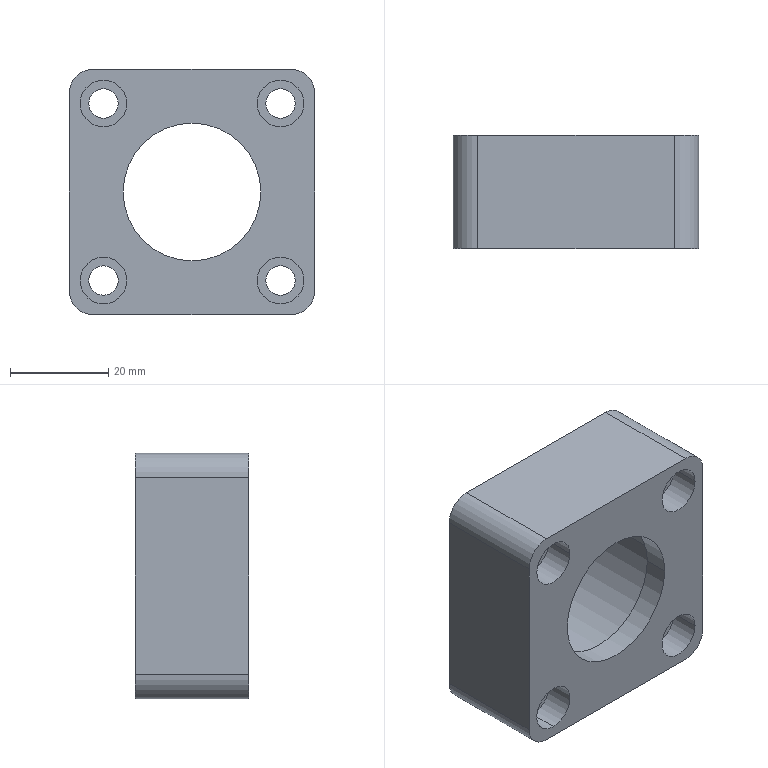Part | NX | features BREP 1 | 1 solid | 35 faces | box 50 x 23 x 50 mm | volume 32986 mm3 | cylinder 24 | plane 11 | commonest cylinder face diameters 6 x8 9.5 x8 10 x4 28 x2 35 x2
STEP:
#1=CARTESIAN_POINT('',(25.,0.,20.));
#2=VERTEX_POINT('',#1);
#3=CARTESIAN_POINT('',(25.,0.,-20.));
#4=VERTEX_POINT('',#3);
#5=CARTESIAN_POINT('',(25.,0.,20.));
#6=DIRECTION('',(0.,0.,-1.));
#7=VECTOR('',#6,1000.);
#8=LINE('',#5,#7);
#9=EDGE_CURVE('',#2,#4,#8,.T.);
#10=ORIENTED_EDGE('',*,*,#9,.F.);
#11=CARTESIAN_POINT('',(20.,0.,25.));
#12=VERTEX_POINT('',#11);
#13=CARTESIAN_POINT('',(20.,0.,20.));
#14=DIRECTION('',(0.,-1.,0.));
#15=DIRECTION('',(1.,0.,0.));
#16=AXIS2_PLACEMENT_3D('',#13,#14,#15);
#17=CIRCLE('',#16,5.);
#18=EDGE_CURVE('',#2,#12,#17,.T.);
#19=ORIENTED_EDGE('',*,*,#18,.T.);
#20=CARTESIAN_POINT('',(-20.,0.,25.));
#21=VERTEX_POINT('',#20);
#22=CARTESIAN_POINT('',(-20.,0.,25.));
#23=DIRECTION('',(1.,0.,0.));
#24=VECTOR('',#23,1000.);
#25=LINE('',#22,#24);
#26=EDGE_CURVE('',#21,#12,#25,.T.);
#27=ORIENTED_EDGE('',*,*,#26,.F.);
#28=CARTESIAN_POINT('',(-25.,0.,20.));
#29=VERTEX_POINT('',#28);
#30=CARTESIAN_POINT('',(-20.,0.,20.));
#31=DIRECTION('',(0.,-1.,0.));
#32=DIRECTION('',(0.,0.,1.));
#33=AXIS2_PLACEMENT_3D('',#30,#31,#32);
#34=CIRCLE('',#33,5.);
#35=EDGE_CURVE('',#21,#29,#34,.T.);
#36=ORIENTED_EDGE('',*,*,#35,.T.);
#37=CARTESIAN_POINT('',(-25.,0.,-20.));
#38=VERTEX_POINT('',#37);
#39=CARTESIAN_POINT('',(-25.,0.,-20.));
#40=DIRECTION('',(0.,0.,1.));
#41=VECTOR('',#40,1000.);
#42=LINE('',#39,#41);
#43=EDGE_CURVE('',#38,#29,#42,.T.);
#44=ORIENTED_EDGE('',*,*,#43,.F.);
#45=CARTESIAN_POINT('',(-20.,0.,-25.));
#46=VERTEX_POINT('',#45);
#47=CARTESIAN_POINT('',(-20.,0.,-20.));
#48=DIRECTION('',(0.,-1.,0.));
#49=DIRECTION('',(-1.,0.,0.));
#50=AXIS2_PLACEMENT_3D('',#47,#48,#49);
#51=CIRCLE('',#50,5.);
#52=EDGE_CURVE('',#38,#46,#51,.T.);
#53=ORIENTED_EDGE('',*,*,#52,.T.);
#54=CARTESIAN_POINT('',(20.,0.,-25.));
#55=VERTEX_POINT('',#54);
#56=CARTESIAN_POINT('',(20.,0.,-25.));
#57=DIRECTION('',(-1.,0.,0.));
#58=VECTOR('',#57,1000.);
#59=LINE('',#56,#58);
#60=EDGE_CURVE('',#55,#46,#59,.T.);
#61=ORIENTED_EDGE('',*,*,#60,.F.);
#62=CARTESIAN_POINT('',(20.,0.,-20.));
#63=DIRECTION('',(0.,-1.,0.));
#64=DIRECTION('',(0.,0.,-1.));
#65=AXIS2_PLACEMENT_3D('',#62,#63,#64);
#66=CIRCLE('',#65,5.);
#67=EDGE_CURVE('',#55,#4,#66,.T.);
#68=ORIENTED_EDGE('',*,*,#67,.T.);
#69=EDGE_LOOP('',(#10,#19,#27,#36,#44,#53,#61,#68));
#70=FACE_BOUND('',#69,.T.);
#71=CARTESIAN_POINT('',(22.75,0.,-18.));
#72=VERTEX_POINT('',#71);
#73=CARTESIAN_POINT('',(13.25,0.,-18.));
#74=VERTEX_POINT('',#73);
#75=CARTESIAN_POINT('',(18.,0.,-18.));
#76=DIRECTION('',(0.,-1.,0.));
#77=DIRECTION('',(1.,0.,0.));
#78=AXIS2_PLACEMENT_3D('',#75,#76,#77);
#79=CIRCLE('',#78,4.75);
#80=EDGE_CURVE('',#72,#74,#79,.T.);
#81=ORIENTED_EDGE('',*,*,#80,.F.);
#82=CARTESIAN_POINT('',(18.,0.,-18.));
#83=DIRECTION('',(0.,-1.,0.));
#84=DIRECTION('',(-1.,0.,0.));
#85=AXIS2_PLACEMENT_3D('',#82,#83,#84);
#86=CIRCLE('',#85,4.75);
#87=EDGE_CURVE('',#74,#72,#86,.T.);
#88=ORIENTED_EDGE('',*,*,#87,.F.);
#89=EDGE_LOOP('',(#81,#88));
#90=FACE_BOUND('',#89,.T.);
#91=CARTESIAN_POINT('',(-18.,0.,-22.75));
#92=VERTEX_POINT('',#91);
#93=CARTESIAN_POINT('',(-18.,0.,-13.25));
#94=VERTEX_POINT('',#93);
#95=CARTESIAN_POINT('',(-18.,0.,-18.));
#96=DIRECTION('',(0.,-1.,0.));
#97=DIRECTION('',(0.,0.,-1.));
#98=AXIS2_PLACEMENT_3D('',#95,#96,#97);
#99=CIRCLE('',#98,4.75);
#100=EDGE_CURVE('',#92,#94,#99,.T.);
#101=ORIENTED_EDGE('',*,*,#100,.F.);
#102=CARTESIAN_POINT('',(-18.,0.,-18.));
#103=DIRECTION('',(0.,-1.,0.));
#104=DIRECTION('',(0.,0.,1.));
#105=AXIS2_PLACEMENT_3D('',#102,#103,#104);
#106=CIRCLE('',#105,4.75);
#107=EDGE_CURVE('',#94,#92,#106,.T.);
#108=ORIENTED_EDGE('',*,*,#107,.F.);
#109=EDGE_LOOP('',(#101,#108));
#110=FACE_BOUND('',#109,.T.);
#111=CARTESIAN_POINT('',(-22.75,0.,18.));
#112=VERTEX_POINT('',#111);
#113=CARTESIAN_POINT('',(-13.25,0.,18.));
#114=VERTEX_POINT('',#113);
#115=CARTESIAN_POINT('',(-18.,0.,18.));
#116=DIRECTION('',(0.,-1.,0.));
#117=DIRECTION('',(-1.,0.,0.));
#118=AXIS2_PLACEMENT_3D('',#115,#116,#117);
#119=CIRCLE('',#118,4.75);
#120=EDGE_CURVE('',#112,#114,#119,.T.);
#121=ORIENTED_EDGE('',*,*,#120,.F.);
#122=CARTESIAN_POINT('',(-18.,0.,18.));
#123=DIRECTION('',(0.,-1.,0.));
#124=DIRECTION('',(1.,0.,0.));
#125=AXIS2_PLACEMENT_3D('',#122,#123,#124);
#126=CIRCLE('',#125,4.75);
#127=EDGE_CURVE('',#114,#112,#126,.T.);
#128=ORIENTED_EDGE('',*,*,#127,.F.);
#129=EDGE_LOOP('',(#121,#128));
#130=FACE_BOUND('',#129,.T.);
#131=CARTESIAN_POINT('',(13.25,0.,18.));
#132=VERTEX_POINT('',#131);
#133=CARTESIAN_POINT('',(22.75,0.,18.));
#134=VERTEX_POINT('',#133);
#135=CARTESIAN_POINT('',(18.,0.,18.));
#136=DIRECTION('',(0.,-1.,0.));
#137=DIRECTION('',(-1.,0.,0.));
#138=AXIS2_PLACEMENT_3D('',#135,#136,#137);
#139=CIRCLE('',#138,4.75);
#140=EDGE_CURVE('',#132,#134,#139,.T.);
#141=ORIENTED_EDGE('',*,*,#140,.F.);
#142=CARTESIAN_POINT('',(18.,0.,18.));
#143=DIRECTION('',(0.,-1.,0.));
#144=DIRECTION('',(1.,0.,0.));
#145=AXIS2_PLACEMENT_3D('',#142,#143,#144);
#146=CIRCLE('',#145,4.75);
#147=EDGE_CURVE('',#134,#132,#146,.T.);
#148=ORIENTED_EDGE('',*,*,#147,.F.);
#149=EDGE_LOOP('',(#141,#148));
#150=FACE_BOUND('',#149,.T.);
#151=CARTESIAN_POINT('',(-14.,0.,0.));
#152=VERTEX_POINT('',#151);
#153=CARTESIAN_POINT('',(14.,0.,0.));
#154=VERTEX_POINT('',#153);
#155=CARTESIAN_POINT('',(0.,0.,0.));
#156=DIRECTION('',(0.,1.,0.));
#157=DIRECTION('',(-1.,0.,0.));
#158=AXIS2_PLACEMENT_3D('',#155,#156,#157);
#159=CIRCLE('',#158,14.);
#160=EDGE_CURVE('',#152,#154,#159,.T.);
#161=ORIENTED_EDGE('',*,*,#160,.T.);
#162=CARTESIAN_POINT('',(0.,0.,0.));
#163=DIRECTION('',(0.,1.,0.));
#164=DIRECTION('',(1.,0.,0.));
#165=AXIS2_PLACEMENT_3D('',#162,#163,#164);
#166=CIRCLE('',#165,14.);
#167=EDGE_CURVE('',#154,#152,#166,.T.);
#168=ORIENTED_EDGE('',*,*,#167,.T.);
#169=EDGE_LOOP('',(#161,#168));
#170=FACE_BOUND('',#169,.T.);
#171=CARTESIAN_POINT('',(0.,0.,0.));
#172=DIRECTION('',(0.,1.,0.));
#173=DIRECTION('',(1.,0.,0.));
#174=AXIS2_PLACEMENT_3D('',#171,#172,#173);
#175=PLANE('',#174);
#176=ADVANCED_FACE('',(#70,#90,#110,#130,#150,#170),#175,.F.);
#177=CARTESIAN_POINT('',(-14.,5.,0.));
#178=VERTEX_POINT('',#177);
#179=CARTESIAN_POINT('',(-14.,5.,0.));
#180=DIRECTION('',(0.,-1.,0.));
#181=VECTOR('',#180,1000.);
#182=LINE('',#179,#181);
#183=EDGE_CURVE('',#178,#152,#182,.T.);
#184=ORIENTED_EDGE('',*,*,#183,.T.);
#185=ORIENTED_EDGE('',*,*,#167,.F.);
#186=CARTESIAN_POINT('',(14.,5.,0.));
#187=VERTEX_POINT('',#186);
#188=CARTESIAN_POINT('',(14.,5.,0.));
#189=DIRECTION('',(0.,-1.,0.));
#190=VECTOR('',#189,1000.);
#191=LINE('',#188,#190);
#192=EDGE_CURVE('',#187,#154,#191,.T.);
#193=ORIENTED_EDGE('',*,*,#192,.F.);
#194=CARTESIAN_POINT('',(0.,5.,0.));
#195=DIRECTION('',(0.,1.,0.));
#196=DIRECTION('',(1.,0.,0.));
#197=AXIS2_PLACEMENT_3D('',#194,#195,#196);
#198=CIRCLE('',#197,14.);
#199=EDGE_CURVE('',#187,#178,#198,.T.);
#200=ORIENTED_EDGE('',*,*,#199,.T.);
#201=EDGE_LOOP('',(#184,#185,#193,#200));
#202=FACE_BOUND('',#201,.T.);
#203=CARTESIAN_POINT('',(0.,23.,0.));
#204=DIRECTION('',(0.,1.,0.));
#205=DIRECTION('',(1.,0.,0.));
#206=AXIS2_PLACEMENT_3D('',#203,#204,#205);
#207=CYLINDRICAL_SURFACE('',#206,14.);
#208=ADVANCED_FACE('',(#202),#207,.F.);
#209=CARTESIAN_POINT('',(-17.5,5.,0.));
#210=VERTEX_POINT('',#209);
#211=CARTESIAN_POINT('',(17.5,5.,0.));
#212=VERTEX_POINT('',#211);
#213=CARTESIAN_POINT('',(0.,5.,0.));
#214=DIRECTION('',(0.,1.,0.));
#215=DIRECTION('',(-1.,0.,0.));
#216=AXIS2_PLACEMENT_3D('',#213,#214,#215);
#217=CIRCLE('',#216,17.5);
#218=EDGE_CURVE('',#210,#212,#217,.T.);
#219=ORIENTED_EDGE('',*,*,#218,.T.);
#220=CARTESIAN_POINT('',(0.,5.,0.));
#221=DIRECTION('',(0.,1.,0.));
#222=DIRECTION('',(1.,0.,0.));
#223=AXIS2_PLACEMENT_3D('',#220,#221,#222);
#224=CIRCLE('',#223,17.5);
#225=EDGE_CURVE('',#212,#210,#224,.T.);
#226=ORIENTED_EDGE('',*,*,#225,.T.);
#227=EDGE_LOOP('',(#219,#226));
#228=FACE_BOUND('',#227,.T.);
#229=CARTESIAN_POINT('',(0.,5.,0.));
#230=DIRECTION('',(0.,1.,0.));
#231=DIRECTION('',(-1.,0.,0.));
#232=AXIS2_PLACEMENT_3D('',#229,#230,#231);
#233=CIRCLE('',#232,14.);
#234=EDGE_CURVE('',#178,#187,#233,.T.);
#235=ORIENTED_EDGE('',*,*,#234,.F.);
#236=ORIENTED_EDGE('',*,*,#199,.F.);
#237=EDGE_LOOP('',(#235,#236));
#238=FACE_BOUND('',#237,.T.);
#239=CARTESIAN_POINT('',(0.,5.,0.));
#240=DIRECTION('',(0.,1.,0.));
#241=DIRECTION('',(1.,0.,0.));
#242=AXIS2_PLACEMENT_3D('',#239,#240,#241);
#243=PLANE('',#242);
#244=ADVANCED_FACE('',(#228,#238),#243,.T.);
#245=CARTESIAN_POINT('',(-17.5,23.,0.));
#246=VERTEX_POINT('',#245);
#247=CARTESIAN_POINT('',(-17.5,23.,0.));
#248=DIRECTION('',(0.,-1.,0.));
#249=VECTOR('',#248,1000.);
#250=LINE('',#247,#249);
#251=EDGE_CURVE('',#246,#210,#250,.T.);
#252=ORIENTED_EDGE('',*,*,#251,.T.);
#253=ORIENTED_EDGE('',*,*,#225,.F.);
#254=CARTESIAN_POINT('',(17.5,23.,0.));
#255=VERTEX_POINT('',#254);
#256=CARTESIAN_POINT('',(17.5,23.,0.));
#257=DIRECTION('',(0.,-1.,0.));
#258=VECTOR('',#257,1000.);
#259=LINE('',#256,#258);
#260=EDGE_CURVE('',#255,#212,#259,.T.);
#261=ORIENTED_EDGE('',*,*,#260,.F.);
#262=CARTESIAN_POINT('',(0.,23.,0.));
#263=DIRECTION('',(0.,1.,0.));
#264=DIRECTION('',(1.,0.,0.));
#265=AXIS2_PLACEMENT_3D('',#262,#263,#264);
#266=CIRCLE('',#265,17.5);
#267=EDGE_CURVE('',#255,#246,#266,.T.);
#268=ORIENTED_EDGE('',*,*,#267,.T.);
#269=EDGE_LOOP('',(#252,#253,#261,#268));
#270=FACE_BOUND('',#269,.T.);
#271=CARTESIAN_POINT('',(0.,23.,0.));
#272=DIRECTION('',(0.,1.,0.));
#273=DIRECTION('',(1.,0.,0.));
#274=AXIS2_PLACEMENT_3D('',#271,#272,#273);
#275=CYLINDRICAL_SURFACE('',#274,17.5);
#276=ADVANCED_FACE('',(#270),#275,.F.);
#277=CARTESIAN_POINT('',(20.,23.,-25.));
#278=VERTEX_POINT('',#277);
#279=CARTESIAN_POINT('',(-20.,23.,-25.));
#280=VERTEX_POINT('',#279);
#281=CARTESIAN_POINT('',(20.,23.,-25.));
#282=DIRECTION('',(-1.,0.,0.));
#283=VECTOR('',#282,1000.);
#284=LINE('',#281,#283);
#285=EDGE_CURVE('',#278,#280,#284,.T.);
#286=ORIENTED_EDGE('',*,*,#285,.T.);
#287=CARTESIAN_POINT('',(-25.,23.,-20.));
#288=VERTEX_POINT('',#287);
#289=CARTESIAN_POINT('',(-20.,23.,-20.));
#290=DIRECTION('',(0.,1.,0.));
#291=DIRECTION('',(0.,0.,-1.));
#292=AXIS2_PLACEMENT_3D('',#289,#290,#291);
#293=CIRCLE('',#292,5.);
#294=EDGE_CURVE('',#280,#288,#293,.T.);
#295=ORIENTED_EDGE('',*,*,#294,.T.);
#296=CARTESIAN_POINT('',(-25.,23.,20.));
#297=VERTEX_POINT('',#296);
#298=CARTESIAN_POINT('',(-25.,23.,-20.));
#299=DIRECTION('',(0.,0.,1.));
#300=VECTOR('',#299,1000.);
#301=LINE('',#298,#300);
#302=EDGE_CURVE('',#288,#297,#301,.T.);
#303=ORIENTED_EDGE('',*,*,#302,.T.);
#304=CARTESIAN_POINT('',(-20.,23.,25.));
#305=VERTEX_POINT('',#304);
#306=CARTESIAN_POINT('',(-20.,23.,20.));
#307=DIRECTION('',(0.,1.,0.));
#308=DIRECTION('',(-1.,0.,0.));
#309=AXIS2_PLACEMENT_3D('',#306,#307,#308);
#310=CIRCLE('',#309,5.);
#311=EDGE_CURVE('',#297,#305,#310,.T.);
#312=ORIENTED_EDGE('',*,*,#311,.T.);
#313=CARTESIAN_POINT('',(20.,23.,25.));
#314=VERTEX_POINT('',#313);
#315=CARTESIAN_POINT('',(-20.,23.,25.));
#316=DIRECTION('',(1.,0.,0.));
#317=VECTOR('',#316,1000.);
#318=LINE('',#315,#317);
#319=EDGE_CURVE('',#305,#314,#318,.T.);
#320=ORIENTED_EDGE('',*,*,#319,.T.);
#321=CARTESIAN_POINT('',(25.,23.,20.));
#322=VERTEX_POINT('',#321);
#323=CARTESIAN_POINT('',(20.,23.,20.));
#324=DIRECTION('',(0.,1.,0.));
#325=DIRECTION('',(0.,0.,1.));
#326=AXIS2_PLACEMENT_3D('',#323,#324,#325);
#327=CIRCLE('',#326,5.);
#328=EDGE_CURVE('',#314,#322,#327,.T.);
#329=ORIENTED_EDGE('',*,*,#328,.T.);
#330=CARTESIAN_POINT('',(25.,23.,-20.));
#331=VERTEX_POINT('',#330);
#332=CARTESIAN_POINT('',(25.,23.,20.));
#333=DIRECTION('',(0.,0.,-1.));
#334=VECTOR('',#333,1000.);
#335=LINE('',#332,#334);
#336=EDGE_CURVE('',#322,#331,#335,.T.);
#337=ORIENTED_EDGE('',*,*,#336,.T.);
#338=CARTESIAN_POINT('',(20.,23.,-20.));
#339=DIRECTION('',(0.,1.,0.));
#340=DIRECTION('',(1.,0.,0.));
#341=AXIS2_PLACEMENT_3D('',#338,#339,#340);
#342=CIRCLE('',#341,5.);
#343=EDGE_CURVE('',#331,#278,#342,.T.);
#344=ORIENTED_EDGE('',*,*,#343,.T.);
#345=EDGE_LOOP('',(#286,#295,#303,#312,#320,#329,#337,#344));
#346=FACE_BOUND('',#345,.T.);
#347=CARTESIAN_POINT('',(21.,23.,-18.));
#348=VERTEX_POINT('',#347);
#349=CARTESIAN_POINT('',(15.,23.,-18.));
#350=VERTEX_POINT('',#349);
#351=CARTESIAN_POINT('',(18.,23.,-18.));
#352=DIRECTION('',(0.,-1.,0.));
#353=DIRECTION('',(1.,0.,0.));
#354=AXIS2_PLACEMENT_3D('',#351,#352,#353);
#355=CIRCLE('',#354,3.);
#356=EDGE_CURVE('',#348,#350,#355,.T.);
#357=ORIENTED_EDGE('',*,*,#356,.T.);
#358=CARTESIAN_POINT('',(18.,23.,-18.));
#359=DIRECTION('',(0.,-1.,0.));
#360=DIRECTION('',(-1.,0.,0.));
#361=AXIS2_PLACEMENT_3D('',#358,#359,#360);
#362=CIRCLE('',#361,3.);
#363=EDGE_CURVE('',#350,#348,#362,.T.);
#364=ORIENTED_EDGE('',*,*,#363,.T.);
#365=EDGE_LOOP('',(#357,#364));
#366=FACE_BOUND('',#365,.T.);
#367=CARTESIAN_POINT('',(-18.,23.,-21.));
#368=VERTEX_POINT('',#367);
#369=CARTESIAN_POINT('',(-18.,23.,-15.));
#370=VERTEX_POINT('',#369);
#371=CARTESIAN_POINT('',(-18.,23.,-18.));
#372=DIRECTION('',(0.,-1.,0.));
#373=DIRECTION('',(0.,0.,-1.));
#374=AXIS2_PLACEMENT_3D('',#371,#372,#373);
#375=CIRCLE('',#374,3.);
#376=EDGE_CURVE('',#368,#370,#375,.T.);
#377=ORIENTED_EDGE('',*,*,#376,.T.);
#378=CARTESIAN_POINT('',(-18.,23.,-18.));
#379=DIRECTION('',(0.,-1.,0.));
#380=DIRECTION('',(0.,0.,1.));
#381=AXIS2_PLACEMENT_3D('',#378,#379,#380);
#382=CIRCLE('',#381,3.);
#383=EDGE_CURVE('',#370,#368,#382,.T.);
#384=ORIENTED_EDGE('',*,*,#383,.T.);
#385=EDGE_LOOP('',(#377,#384));
#386=FACE_BOUND('',#385,.T.);
#387=CARTESIAN_POINT('',(-21.,23.,18.));
#388=VERTEX_POINT('',#387);
#389=CARTESIAN_POINT('',(-15.,23.,18.));
#390=VERTEX_POINT('',#389);
#391=CARTESIAN_POINT('',(-18.,23.,18.));
#392=DIRECTION('',(0.,-1.,0.));
#393=DIRECTION('',(-1.,0.,0.));
#394=AXIS2_PLACEMENT_3D('',#391,#392,#393);
#395=CIRCLE('',#394,3.);
#396=EDGE_CURVE('',#388,#390,#395,.T.);
#397=ORIENTED_EDGE('',*,*,#396,.T.);
#398=CARTESIAN_POINT('',(-18.,23.,18.));
#399=DIRECTION('',(0.,-1.,0.));
#400=DIRECTION('',(1.,0.,0.));
#401=AXIS2_PLACEMENT_3D('',#398,#399,#400);
#402=CIRCLE('',#401,3.);
#403=EDGE_CURVE('',#390,#388,#402,.T.);
#404=ORIENTED_EDGE('',*,*,#403,.T.);
#405=EDGE_LOOP('',(#397,#404));
#406=FACE_BOUND('',#405,.T.);
#407=CARTESIAN_POINT('',(15.,23.,18.));
#408=VERTEX_POINT('',#407);
#409=CARTESIAN_POINT('',(21.,23.,18.));
#410=VERTEX_POINT('',#409);
#411=CARTESIAN_POINT('',(18.,23.,18.));
#412=DIRECTION('',(0.,-1.,0.));
#413=DIRECTION('',(-1.,0.,0.));
#414=AXIS2_PLACEMENT_3D('',#411,#412,#413);
#415=CIRCLE('',#414,3.);
#416=EDGE_CURVE('',#408,#410,#415,.T.);
#417=ORIENTED_EDGE('',*,*,#416,.T.);
#418=CARTESIAN_POINT('',(18.,23.,18.));
#419=DIRECTION('',(0.,-1.,0.));
#420=DIRECTION('',(1.,0.,0.));
#421=AXIS2_PLACEMENT_3D('',#418,#419,#420);
#422=CIRCLE('',#421,3.);
#423=EDGE_CURVE('',#410,#408,#422,.T.);
#424=ORIENTED_EDGE('',*,*,#423,.T.);
#425=EDGE_LOOP('',(#417,#424));
#426=FACE_BOUND('',#425,.T.);
#427=CARTESIAN_POINT('',(0.,23.,0.));
#428=DIRECTION('',(0.,1.,0.));
#429=DIRECTION('',(-1.,0.,0.));
#430=AXIS2_PLACEMENT_3D('',#427,#428,#429);
#431=CIRCLE('',#430,17.5);
#432=EDGE_CURVE('',#246,#255,#431,.T.);
#433=ORIENTED_EDGE('',*,*,#432,.F.);
#434=ORIENTED_EDGE('',*,*,#267,.F.);
#435=EDGE_LOOP('',(#433,#434));
#436=FACE_BOUND('',#435,.T.);
#437=CARTESIAN_POINT('',(0.,23.,0.));
#438=DIRECTION('',(0.,1.,0.));
#439=DIRECTION('',(1.,0.,0.));
#440=AXIS2_PLACEMENT_3D('',#437,#438,#439);
#441=PLANE('',#440);
#442=ADVANCED_FACE('',(#346,#366,#386,#406,#426,#436),#441,.T.);
#443=ORIENTED_EDGE('',*,*,#260,.T.);
#444=ORIENTED_EDGE('',*,*,#218,.F.);
#445=ORIENTED_EDGE('',*,*,#251,.F.);
#446=ORIENTED_EDGE('',*,*,#432,.T.);
#447=EDGE_LOOP('',(#443,#444,#445,#446));
#448=FACE_BOUND('',#447,.T.);
#449=CARTESIAN_POINT('',(0.,23.,0.));
#450=DIRECTION('',(0.,1.,0.));
#451=DIRECTION('',(1.,0.,0.));
#452=AXIS2_PLACEMENT_3D('',#449,#450,#451);
#453=CYLINDRICAL_SURFACE('',#452,17.5);
#454=ADVANCED_FACE('',(#448),#453,.F.);
#455=CARTESIAN_POINT('',(15.,6.,-18.));
#456=VERTEX_POINT('',#455);
#457=CARTESIAN_POINT('',(15.,23.,-18.));
#458=DIRECTION('',(0.,-1.,0.));
#459=VECTOR('',#458,1000.);
#460=LINE('',#457,#459);
#461=EDGE_CURVE('',#350,#456,#460,.T.);
#462=ORIENTED_EDGE('',*,*,#461,.T.);
#463=CARTESIAN_POINT('',(21.,6.,-18.));
#464=VERTEX_POINT('',#463);
#465=CARTESIAN_POINT('',(18.,6.,-18.));
#466=DIRECTION('',(0.,-1.,0.));
#467=DIRECTION('',(-1.,0.,0.));
#468=AXIS2_PLACEMENT_3D('',#465,#466,#467);
#469=CIRCLE('',#468,3.);
#470=EDGE_CURVE('',#456,#464,#469,.T.);
#471=ORIENTED_EDGE('',*,*,#470,.T.);
#472=CARTESIAN_POINT('',(21.,23.,-18.));
#473=DIRECTION('',(0.,-1.,0.));
#474=VECTOR('',#473,1000.);
#475=LINE('',#472,#474);
#476=EDGE_CURVE('',#348,#464,#475,.T.);
#477=ORIENTED_EDGE('',*,*,#476,.F.);
#478=ORIENTED_EDGE('',*,*,#363,.F.);
#479=EDGE_LOOP('',(#462,#471,#477,#478));
#480=FACE_BOUND('',#479,.T.);
#481=CARTESIAN_POINT('',(18.,33.393,-18.));
#482=DIRECTION('',(0.,-1.,0.));
#483=DIRECTION('',(-1.,0.,0.));
#484=AXIS2_PLACEMENT_3D('',#481,#482,#483);
#485=CYLINDRICAL_SURFACE('',#484,3.);
#486=ADVANCED_FACE('',(#480),#485,.F.);
#487=ORIENTED_EDGE('',*,*,#476,.T.);
#488=CARTESIAN_POINT('',(18.,6.,-18.));
#489=DIRECTION('',(0.,1.,0.));
#490=DIRECTION('',(-1.,0.,0.));
#491=AXIS2_PLACEMENT_3D('',#488,#489,#490);
#492=CIRCLE('',#491,3.);
#493=EDGE_CURVE('',#456,#464,#492,.T.);
#494=ORIENTED_EDGE('',*,*,#493,.F.);
#495=ORIENTED_EDGE('',*,*,#461,.F.);
#496=ORIENTED_EDGE('',*,*,#356,.F.);
#497=EDGE_LOOP('',(#487,#494,#495,#496));
#498=FACE_BOUND('',#497,.T.);
#499=CARTESIAN_POINT('',(18.,33.393,-18.));
#500=DIRECTION('',(0.,-1.,0.));
#501=DIRECTION('',(-1.,0.,0.));
#502=AXIS2_PLACEMENT_3D('',#499,#500,#501);
#503=CYLINDRICAL_SURFACE('',#502,3.);
#504=ADVANCED_FACE('',(#498),#503,.F.);
#505=CARTESIAN_POINT('',(13.25,6.,-18.));
#506=VERTEX_POINT('',#505);
#507=CARTESIAN_POINT('',(22.75,6.,-18.));
#508=VERTEX_POINT('',#507);
#509=CARTESIAN_POINT('',(18.,6.,-18.));
#510=DIRECTION('',(0.,1.,0.));
#511=DIRECTION('',(-1.,0.,0.));
#512=AXIS2_PLACEMENT_3D('',#509,#510,#511);
#513=CIRCLE('',#512,4.75);
#514=EDGE_CURVE('',#506,#508,#513,.T.);
#515=ORIENTED_EDGE('',*,*,#514,.F.);
#516=CARTESIAN_POINT('',(18.,6.,-18.));
#517=DIRECTION('',(0.,-1.,0.));
#518=DIRECTION('',(-1.,0.,0.));
#519=AXIS2_PLACEMENT_3D('',#516,#517,#518);
#520=CIRCLE('',#519,4.75);
#521=EDGE_CURVE('',#506,#508,#520,.T.);
#522=ORIENTED_EDGE('',*,*,#521,.T.);
#523=EDGE_LOOP('',(#515,#522));
#524=FACE_BOUND('',#523,.T.);
#525=ORIENTED_EDGE('',*,*,#470,.F.);
#526=ORIENTED_EDGE('',*,*,#493,.T.);
#527=EDGE_LOOP('',(#525,#526));
#528=FACE_BOUND('',#527,.T.);
#529=CARTESIAN_POINT('',(18.,6.,-18.));
#530=DIRECTION('',(0.,-1.,0.));
#531=DIRECTION('',(0.,0.,-1.));
#532=AXIS2_PLACEMENT_3D('',#529,#530,#531);
#533=PLANE('',#532);
#534=ADVANCED_FACE('',(#524,#528),#533,.T.);
#535=CARTESIAN_POINT('',(22.75,6.,-18.));
#536=DIRECTION('',(0.,-1.,0.));
#537=VECTOR('',#536,1000.);
#538=LINE('',#535,#537);
#539=EDGE_CURVE('',#72,#508,#538,.F.);
#540=ORIENTED_EDGE('',*,*,#539,.T.);
#541=ORIENTED_EDGE('',*,*,#521,.F.);
#542=CARTESIAN_POINT('',(13.25,6.,-18.));
#543=DIRECTION('',(0.,-1.,0.));
#544=VECTOR('',#543,1000.);
#545=LINE('',#542,#544);
#546=EDGE_CURVE('',#74,#506,#545,.F.);
#547=ORIENTED_EDGE('',*,*,#546,.F.);
#548=ORIENTED_EDGE('',*,*,#87,.T.);
#549=EDGE_LOOP('',(#540,#541,#547,#548));
#550=FACE_BOUND('',#549,.T.);
#551=CARTESIAN_POINT('',(18.,33.393,-18.));
#552=DIRECTION('',(0.,-1.,0.));
#553=DIRECTION('',(-1.,0.,0.));
#554=AXIS2_PLACEMENT_3D('',#551,#552,#553);
#555=CYLINDRICAL_SURFACE('',#554,4.75);
#556=ADVANCED_FACE('',(#550),#555,.F.);
#557=ORIENTED_EDGE('',*,*,#546,.T.);
#558=ORIENTED_EDGE('',*,*,#514,.T.);
#559=ORIENTED_EDGE('',*,*,#539,.F.);
#560=ORIENTED_EDGE('',*,*,#80,.T.);
#561=EDGE_LOOP('',(#557,#558,#559,#560));
#562=FACE_BOUND('',#561,.T.);
#563=CARTESIAN_POINT('',(18.,33.393,-18.));
#564=DIRECTION('',(0.,-1.,0.));
#565=DIRECTION('',(-1.,0.,0.));
#566=AXIS2_PLACEMENT_3D('',#563,#564,#565);
#567=CYLINDRICAL_SURFACE('',#566,4.75);
#568=ADVANCED_FACE('',(#562),#567,.F.);
#569=CARTESIAN_POINT('',(-18.,6.,-15.));
#570=VERTEX_POINT('',#569);
#571=CARTESIAN_POINT('',(-18.,23.,-15.));
#572=DIRECTION('',(0.,-1.,0.));
#573=VECTOR('',#572,1000.);
#574=LINE('',#571,#573);
#575=EDGE_CURVE('',#570,#370,#574,.F.);
#576=ORIENTED_EDGE('',*,*,#575,.F.);
#577=CARTESIAN_POINT('',(-18.,6.,-21.));
#578=VERTEX_POINT('',#577);
#579=CARTESIAN_POINT('',(-18.,6.,-18.));
#580=DIRECTION('',(0.,-1.,0.));
#581=DIRECTION('',(0.,0.,1.));
#582=AXIS2_PLACEMENT_3D('',#579,#580,#581);
#583=CIRCLE('',#582,3.);
#584=EDGE_CURVE('',#570,#578,#583,.T.);
#585=ORIENTED_EDGE('',*,*,#584,.T.);
#586=CARTESIAN_POINT('',(-18.,23.,-21.));
#587=DIRECTION('',(0.,-1.,0.));
#588=VECTOR('',#587,1000.);
#589=LINE('',#586,#588);
#590=EDGE_CURVE('',#578,#368,#589,.F.);
#591=ORIENTED_EDGE('',*,*,#590,.T.);
#592=ORIENTED_EDGE('',*,*,#383,.F.);
#593=EDGE_LOOP('',(#576,#585,#591,#592));
#594=FACE_BOUND('',#593,.T.);
#595=CARTESIAN_POINT('',(-18.,33.393,-18.));
#596=DIRECTION('',(0.,-1.,0.));
#597=DIRECTION('',(0.,0.,1.));
#598=AXIS2_PLACEMENT_3D('',#595,#596,#597);
#599=CYLINDRICAL_SURFACE('',#598,3.);
#600=ADVANCED_FACE('',(#594),#599,.F.);
#601=ORIENTED_EDGE('',*,*,#590,.F.);
#602=CARTESIAN_POINT('',(-18.,6.,-18.));
#603=DIRECTION('',(0.,1.,0.));
#604=DIRECTION('',(0.,0.,1.));
#605=AXIS2_PLACEMENT_3D('',#602,#603,#604);
#606=CIRCLE('',#605,3.);
#607=EDGE_CURVE('',#570,#578,#606,.T.);
#608=ORIENTED_EDGE('',*,*,#607,.F.);
#609=ORIENTED_EDGE('',*,*,#575,.T.);
#610=ORIENTED_EDGE('',*,*,#376,.F.);
#611=EDGE_LOOP('',(#601,#608,#609,#610));
#612=FACE_BOUND('',#611,.T.);
#613=CARTESIAN_POINT('',(-18.,33.393,-18.));
#614=DIRECTION('',(0.,-1.,0.));
#615=DIRECTION('',(0.,0.,1.));
#616=AXIS2_PLACEMENT_3D('',#613,#614,#615);
#617=CYLINDRICAL_SURFACE('',#616,3.);
#618=ADVANCED_FACE('',(#612),#617,.F.);
#619=CARTESIAN_POINT('',(-18.,6.,-13.25));
#620=VERTEX_POINT('',#619);
#621=CARTESIAN_POINT('',(-18.,6.,-22.75));
#622=VERTEX_POINT('',#621);
#623=CARTESIAN_POINT('',(-18.,6.,-18.));
#624=DIRECTION('',(0.,1.,0.));
#625=DIRECTION('',(0.,0.,1.));
#626=AXIS2_PLACEMENT_3D('',#623,#624,#625);
#627=CIRCLE('',#626,4.75);
#628=EDGE_CURVE('',#620,#622,#627,.T.);
#629=ORIENTED_EDGE('',*,*,#628,.F.);
#630=CARTESIAN_POINT('',(-18.,6.,-18.));
#631=DIRECTION('',(0.,-1.,0.));
#632=DIRECTION('',(0.,0.,1.));
#633=AXIS2_PLACEMENT_3D('',#630,#631,#632);
#634=CIRCLE('',#633,4.75);
#635=EDGE_CURVE('',#620,#622,#634,.T.);
#636=ORIENTED_EDGE('',*,*,#635,.T.);
#637=EDGE_LOOP('',(#629,#636));
#638=FACE_BOUND('',#637,.T.);
#639=ORIENTED_EDGE('',*,*,#584,.F.);
#640=ORIENTED_EDGE('',*,*,#607,.T.);
#641=EDGE_LOOP('',(#639,#640));
#642=FACE_BOUND('',#641,.T.);
#643=CARTESIAN_POINT('',(-18.,6.,-18.));
#644=DIRECTION('',(0.,-1.,0.));
#645=DIRECTION('',(0.,0.,-1.));
#646=AXIS2_PLACEMENT_3D('',#643,#644,#645);
#647=PLANE('',#646);
#648=ADVANCED_FACE('',(#638,#642),#647,.T.);
#649=CARTESIAN_POINT('',(-18.,6.,-22.75));
#650=DIRECTION('',(0.,-1.,0.));
#651=VECTOR('',#650,1000.);
#652=LINE('',#649,#651);
#653=EDGE_CURVE('',#622,#92,#652,.T.);
#654=ORIENTED_EDGE('',*,*,#653,.F.);
#655=ORIENTED_EDGE('',*,*,#635,.F.);
#656=CARTESIAN_POINT('',(-18.,6.,-13.25));
#657=DIRECTION('',(0.,-1.,0.));
#658=VECTOR('',#657,1000.);
#659=LINE('',#656,#658);
#660=EDGE_CURVE('',#620,#94,#659,.T.);
#661=ORIENTED_EDGE('',*,*,#660,.T.);
#662=ORIENTED_EDGE('',*,*,#107,.T.);
#663=EDGE_LOOP('',(#654,#655,#661,#662));
#664=FACE_BOUND('',#663,.T.);
#665=CARTESIAN_POINT('',(-18.,33.393,-18.));
#666=DIRECTION('',(0.,-1.,0.));
#667=DIRECTION('',(0.,0.,1.));
#668=AXIS2_PLACEMENT_3D('',#665,#666,#667);
#669=CYLINDRICAL_SURFACE('',#668,4.75);
#670=ADVANCED_FACE('',(#664),#669,.F.);
#671=ORIENTED_EDGE('',*,*,#660,.F.);
#672=ORIENTED_EDGE('',*,*,#628,.T.);
#673=ORIENTED_EDGE('',*,*,#653,.T.);
#674=ORIENTED_EDGE('',*,*,#100,.T.);
#675=EDGE_LOOP('',(#671,#672,#673,#674));
#676=FACE_BOUND('',#675,.T.);
#677=CARTESIAN_POINT('',(-18.,33.393,-18.));
#678=DIRECTION('',(0.,-1.,0.));
#679=DIRECTION('',(0.,0.,1.));
#680=AXIS2_PLACEMENT_3D('',#677,#678,#679);
#681=CYLINDRICAL_SURFACE('',#680,4.75);
#682=ADVANCED_FACE('',(#676),#681,.F.);
#683=CARTESIAN_POINT('',(-15.,6.,18.));
#684=VERTEX_POINT('',#683);
#685=CARTESIAN_POINT('',(-15.,23.,18.));
#686=DIRECTION('',(0.,-1.,0.));
#687=VECTOR('',#686,1000.);
#688=LINE('',#685,#687);
#689=EDGE_CURVE('',#684,#390,#688,.F.);
#690=ORIENTED_EDGE('',*,*,#689,.F.);
#691=CARTESIAN_POINT('',(-21.,6.,18.));
#692=VERTEX_POINT('',#691);
#693=CARTESIAN_POINT('',(-18.,6.,18.));
#694=DIRECTION('',(0.,-1.,0.));
#695=DIRECTION('',(1.,0.,0.));
#696=AXIS2_PLACEMENT_3D('',#693,#694,#695);
#697=CIRCLE('',#696,3.);
#698=EDGE_CURVE('',#684,#692,#697,.T.);
#699=ORIENTED_EDGE('',*,*,#698,.T.);
#700=CARTESIAN_POINT('',(-21.,23.,18.));
#701=DIRECTION('',(0.,-1.,0.));
#702=VECTOR('',#701,1000.);
#703=LINE('',#700,#702);
#704=EDGE_CURVE('',#692,#388,#703,.F.);
#705=ORIENTED_EDGE('',*,*,#704,.T.);
#706=ORIENTED_EDGE('',*,*,#403,.F.);
#707=EDGE_LOOP('',(#690,#699,#705,#706));
#708=FACE_BOUND('',#707,.T.);
#709=CARTESIAN_POINT('',(-18.,33.393,18.));
#710=DIRECTION('',(0.,-1.,0.));
#711=DIRECTION('',(1.,0.,0.));
#712=AXIS2_PLACEMENT_3D('',#709,#710,#711);
#713=CYLINDRICAL_SURFACE('',#712,3.);
#714=ADVANCED_FACE('',(#708),#713,.F.);
#715=ORIENTED_EDGE('',*,*,#704,.F.);
#716=CARTESIAN_POINT('',(-18.,6.,18.));
#717=DIRECTION('',(0.,1.,0.));
#718=DIRECTION('',(1.,0.,0.));
#719=AXIS2_PLACEMENT_3D('',#716,#717,#718);
#720=CIRCLE('',#719,3.);
#721=EDGE_CURVE('',#684,#692,#720,.T.);
#722=ORIENTED_EDGE('',*,*,#721,.F.);
#723=ORIENTED_EDGE('',*,*,#689,.T.);
#724=ORIENTED_EDGE('',*,*,#396,.F.);
#725=EDGE_LOOP('',(#715,#722,#723,#724));
#726=FACE_BOUND('',#725,.T.);
#727=CARTESIAN_POINT('',(-18.,33.393,18.));
#728=DIRECTION('',(0.,-1.,0.));
#729=DIRECTION('',(1.,0.,0.));
#730=AXIS2_PLACEMENT_3D('',#727,#728,#729);
#731=CYLINDRICAL_SURFACE('',#730,3.);
#732=ADVANCED_FACE('',(#726),#731,.F.);
#733=CARTESIAN_POINT('',(-13.25,6.,18.));
#734=VERTEX_POINT('',#733);
#735=CARTESIAN_POINT('',(-22.75,6.,18.));
#736=VERTEX_POINT('',#735);
#737=CARTESIAN_POINT('',(-18.,6.,18.));
#738=DIRECTION('',(0.,1.,0.));
#739=DIRECTION('',(1.,0.,0.));
#740=AXIS2_PLACEMENT_3D('',#737,#738,#739);
#741=CIRCLE('',#740,4.75);
#742=EDGE_CURVE('',#734,#736,#741,.T.);
#743=ORIENTED_EDGE('',*,*,#742,.F.);
#744=CARTESIAN_POINT('',(-18.,6.,18.));
#745=DIRECTION('',(0.,-1.,0.));
#746=DIRECTION('',(1.,0.,0.));
#747=AXIS2_PLACEMENT_3D('',#744,#745,#746);
#748=CIRCLE('',#747,4.75);
#749=EDGE_CURVE('',#734,#736,#748,.T.);
#750=ORIENTED_EDGE('',*,*,#749,.T.);
#751=EDGE_LOOP('',(#743,#750));
#752=FACE_BOUND('',#751,.T.);
#753=ORIENTED_EDGE('',*,*,#698,.F.);
#754=ORIENTED_EDGE('',*,*,#721,.T.);
#755=EDGE_LOOP('',(#753,#754));
#756=FACE_BOUND('',#755,.T.);
#757=CARTESIAN_POINT('',(-18.,6.,18.));
#758=DIRECTION('',(0.,-1.,0.));
#759=DIRECTION('',(0.,0.,-1.));
#760=AXIS2_PLACEMENT_3D('',#757,#758,#759);
#761=PLANE('',#760);
#762=ADVANCED_FACE('',(#752,#756),#761,.T.);
#763=CARTESIAN_POINT('',(-22.75,6.,18.));
#764=DIRECTION('',(0.,-1.,0.));
#765=VECTOR('',#764,1000.);
#766=LINE('',#763,#765);
#767=EDGE_CURVE('',#736,#112,#766,.T.);
#768=ORIENTED_EDGE('',*,*,#767,.F.);
#769=ORIENTED_EDGE('',*,*,#749,.F.);
#770=CARTESIAN_POINT('',(-13.25,6.,18.));
#771=DIRECTION('',(0.,-1.,0.));
#772=VECTOR('',#771,1000.);
#773=LINE('',#770,#772);
#774=EDGE_CURVE('',#734,#114,#773,.T.);
#775=ORIENTED_EDGE('',*,*,#774,.T.);
#776=ORIENTED_EDGE('',*,*,#127,.T.);
#777=EDGE_LOOP('',(#768,#769,#775,#776));
#778=FACE_BOUND('',#777,.T.);
#779=CARTESIAN_POINT('',(-18.,33.393,18.));
#780=DIRECTION('',(0.,-1.,0.));
#781=DIRECTION('',(1.,0.,0.));
#782=AXIS2_PLACEMENT_3D('',#779,#780,#781);
#783=CYLINDRICAL_SURFACE('',#782,4.75);
#784=ADVANCED_FACE('',(#778),#783,.F.);
#785=ORIENTED_EDGE('',*,*,#774,.F.);
#786=ORIENTED_EDGE('',*,*,#742,.T.);
#787=ORIENTED_EDGE('',*,*,#767,.T.);
#788=ORIENTED_EDGE('',*,*,#120,.T.);
#789=EDGE_LOOP('',(#785,#786,#787,#788));
#790=FACE_BOUND('',#789,.T.);
#791=CARTESIAN_POINT('',(-18.,33.393,18.));
#792=DIRECTION('',(0.,-1.,0.));
#793=DIRECTION('',(1.,0.,0.));
#794=AXIS2_PLACEMENT_3D('',#791,#792,#793);
#795=CYLINDRICAL_SURFACE('',#794,4.75);
#796=ADVANCED_FACE('',(#790),#795,.F.);
#797=CARTESIAN_POINT('',(21.,6.,18.));
#798=VERTEX_POINT('',#797);
#799=CARTESIAN_POINT('',(21.,23.,18.));
#800=DIRECTION('',(0.,-1.,0.));
#801=VECTOR('',#800,1000.);
#802=LINE('',#799,#801);
#803=EDGE_CURVE('',#798,#410,#802,.F.);
#804=ORIENTED_EDGE('',*,*,#803,.F.);
#805=CARTESIAN_POINT('',(15.,6.,18.));
#806=VERTEX_POINT('',#805);
#807=CARTESIAN_POINT('',(18.,6.,18.));
#808=DIRECTION('',(0.,-1.,0.));
#809=DIRECTION('',(1.,0.,0.));
#810=AXIS2_PLACEMENT_3D('',#807,#808,#809);
#811=CIRCLE('',#810,3.);
#812=EDGE_CURVE('',#798,#806,#811,.T.);
#813=ORIENTED_EDGE('',*,*,#812,.T.);
#814=CARTESIAN_POINT('',(15.,23.,18.));
#815=DIRECTION('',(0.,-1.,0.));
#816=VECTOR('',#815,1000.);
#817=LINE('',#814,#816);
#818=EDGE_CURVE('',#806,#408,#817,.F.);
#819=ORIENTED_EDGE('',*,*,#818,.T.);
#820=ORIENTED_EDGE('',*,*,#423,.F.);
#821=EDGE_LOOP('',(#804,#813,#819,#820));
#822=FACE_BOUND('',#821,.T.);
#823=CARTESIAN_POINT('',(18.,33.393,18.));
#824=DIRECTION('',(0.,-1.,0.));
#825=DIRECTION('',(1.,0.,0.));
#826=AXIS2_PLACEMENT_3D('',#823,#824,#825);
#827=CYLINDRICAL_SURFACE('',#826,3.);
#828=ADVANCED_FACE('',(#822),#827,.F.);
#829=ORIENTED_EDGE('',*,*,#818,.F.);
#830=CARTESIAN_POINT('',(18.,6.,18.));
#831=DIRECTION('',(0.,1.,0.));
#832=DIRECTION('',(1.,0.,0.));
#833=AXIS2_PLACEMENT_3D('',#830,#831,#832);
#834=CIRCLE('',#833,3.);
#835=EDGE_CURVE('',#798,#806,#834,.T.);
#836=ORIENTED_EDGE('',*,*,#835,.F.);
#837=ORIENTED_EDGE('',*,*,#803,.T.);
#838=ORIENTED_EDGE('',*,*,#416,.F.);
#839=EDGE_LOOP('',(#829,#836,#837,#838));
#840=FACE_BOUND('',#839,.T.);
#841=CARTESIAN_POINT('',(18.,33.393,18.));
#842=DIRECTION('',(0.,-1.,0.));
#843=DIRECTION('',(1.,0.,0.));
#844=AXIS2_PLACEMENT_3D('',#841,#842,#843);
#845=CYLINDRICAL_SURFACE('',#844,3.);
#846=ADVANCED_FACE('',(#840),#845,.F.);
#847=CARTESIAN_POINT('',(22.75,6.,18.));
#848=VERTEX_POINT('',#847);
#849=CARTESIAN_POINT('',(13.25,6.,18.));
#850=VERTEX_POINT('',#849);
#851=CARTESIAN_POINT('',(18.,6.,18.));
#852=DIRECTION('',(0.,1.,0.));
#853=DIRECTION('',(1.,0.,0.));
#854=AXIS2_PLACEMENT_3D('',#851,#852,#853);
#855=CIRCLE('',#854,4.75);
#856=EDGE_CURVE('',#848,#850,#855,.T.);
#857=ORIENTED_EDGE('',*,*,#856,.F.);
#858=CARTESIAN_POINT('',(18.,6.,18.));
#859=DIRECTION('',(0.,-1.,0.));
#860=DIRECTION('',(1.,0.,0.));
#861=AXIS2_PLACEMENT_3D('',#858,#859,#860);
#862=CIRCLE('',#861,4.75);
#863=EDGE_CURVE('',#848,#850,#862,.T.);
#864=ORIENTED_EDGE('',*,*,#863,.T.);
#865=EDGE_LOOP('',(#857,#864));
#866=FACE_BOUND('',#865,.T.);
#867=ORIENTED_EDGE('',*,*,#812,.F.);
#868=ORIENTED_EDGE('',*,*,#835,.T.);
#869=EDGE_LOOP('',(#867,#868));
#870=FACE_BOUND('',#869,.T.);
#871=CARTESIAN_POINT('',(18.,6.,18.));
#872=DIRECTION('',(0.,-1.,0.));
#873=DIRECTION('',(0.,0.,-1.));
#874=AXIS2_PLACEMENT_3D('',#871,#872,#873);
#875=PLANE('',#874);
#876=ADVANCED_FACE('',(#866,#870),#875,.T.);
#877=CARTESIAN_POINT('',(13.25,6.,18.));
#878=DIRECTION('',(0.,-1.,0.));
#879=VECTOR('',#878,1000.);
#880=LINE('',#877,#879);
#881=EDGE_CURVE('',#850,#132,#880,.T.);
#882=ORIENTED_EDGE('',*,*,#881,.F.);
#883=ORIENTED_EDGE('',*,*,#863,.F.);
#884=CARTESIAN_POINT('',(22.75,6.,18.));
#885=DIRECTION('',(0.,-1.,0.));
#886=VECTOR('',#885,1000.);
#887=LINE('',#884,#886);
#888=EDGE_CURVE('',#848,#134,#887,.T.);
#889=ORIENTED_EDGE('',*,*,#888,.T.);
#890=ORIENTED_EDGE('',*,*,#147,.T.);
#891=EDGE_LOOP('',(#882,#883,#889,#890));
#892=FACE_BOUND('',#891,.T.);
#893=CARTESIAN_POINT('',(18.,33.393,18.));
#894=DIRECTION('',(0.,-1.,0.));
#895=DIRECTION('',(1.,0.,0.));
#896=AXIS2_PLACEMENT_3D('',#893,#894,#895);
#897=CYLINDRICAL_SURFACE('',#896,4.75);
#898=ADVANCED_FACE('',(#892),#897,.F.);
#899=ORIENTED_EDGE('',*,*,#888,.F.);
#900=ORIENTED_EDGE('',*,*,#856,.T.);
#901=ORIENTED_EDGE('',*,*,#881,.T.);
#902=ORIENTED_EDGE('',*,*,#140,.T.);
#903=EDGE_LOOP('',(#899,#900,#901,#902));
#904=FACE_BOUND('',#903,.T.);
#905=CARTESIAN_POINT('',(18.,33.393,18.));
#906=DIRECTION('',(0.,-1.,0.));
#907=DIRECTION('',(1.,0.,0.));
#908=AXIS2_PLACEMENT_3D('',#905,#906,#907);
#909=CYLINDRICAL_SURFACE('',#908,4.75);
#910=ADVANCED_FACE('',(#904),#909,.F.);
#911=CARTESIAN_POINT('',(20.,23.,-25.));
#912=DIRECTION('',(0.,-1.,0.));
#913=VECTOR('',#912,1000.);
#914=LINE('',#911,#913);
#915=EDGE_CURVE('',#278,#55,#914,.T.);
#916=ORIENTED_EDGE('',*,*,#915,.F.);
#917=ORIENTED_EDGE('',*,*,#343,.F.);
#918=CARTESIAN_POINT('',(25.,23.,-20.));
#919=DIRECTION('',(0.,-1.,0.));
#920=VECTOR('',#919,1000.);
#921=LINE('',#918,#920);
#922=EDGE_CURVE('',#331,#4,#921,.T.);
#923=ORIENTED_EDGE('',*,*,#922,.T.);
#924=ORIENTED_EDGE('',*,*,#67,.F.);
#925=EDGE_LOOP('',(#916,#917,#923,#924));
#926=FACE_BOUND('',#925,.T.);
#927=CARTESIAN_POINT('',(20.,52.983,-20.));
#928=DIRECTION('',(0.,-1.,0.));
#929=DIRECTION('',(0.,0.,-1.));
#930=AXIS2_PLACEMENT_3D('',#927,#928,#929);
#931=CYLINDRICAL_SURFACE('',#930,5.);
#932=ADVANCED_FACE('',(#926),#931,.T.);
#933=ORIENTED_EDGE('',*,*,#336,.F.);
#934=CARTESIAN_POINT('',(25.,23.,20.));
#935=DIRECTION('',(0.,-1.,0.));
#936=VECTOR('',#935,1000.);
#937=LINE('',#934,#936);
#938=EDGE_CURVE('',#322,#2,#937,.T.);
#939=ORIENTED_EDGE('',*,*,#938,.T.);
#940=ORIENTED_EDGE('',*,*,#9,.T.);
#941=ORIENTED_EDGE('',*,*,#922,.F.);
#942=EDGE_LOOP('',(#933,#939,#940,#941));
#943=FACE_BOUND('',#942,.T.);
#944=CARTESIAN_POINT('',(25.,0.,25.));
#945=DIRECTION('',(1.,0.,0.));
#946=DIRECTION('',(0.,1.,0.));
#947=AXIS2_PLACEMENT_3D('',#944,#945,#946);
#948=PLANE('',#947);
#949=ADVANCED_FACE('',(#943),#948,.T.);
#950=ORIENTED_EDGE('',*,*,#938,.F.);
#951=ORIENTED_EDGE('',*,*,#328,.F.);
#952=CARTESIAN_POINT('',(20.,23.,25.));
#953=DIRECTION('',(0.,-1.,0.));
#954=VECTOR('',#953,1000.);
#955=LINE('',#952,#954);
#956=EDGE_CURVE('',#314,#12,#955,.T.);
#957=ORIENTED_EDGE('',*,*,#956,.T.);
#958=ORIENTED_EDGE('',*,*,#18,.F.);
#959=EDGE_LOOP('',(#950,#951,#957,#958));
#960=FACE_BOUND('',#959,.T.);
#961=CARTESIAN_POINT('',(20.,52.983,20.));
#962=DIRECTION('',(0.,-1.,0.));
#963=DIRECTION('',(1.,0.,0.));
#964=AXIS2_PLACEMENT_3D('',#961,#962,#963);
#965=CYLINDRICAL_SURFACE('',#964,5.);
#966=ADVANCED_FACE('',(#960),#965,.T.);
#967=ORIENTED_EDGE('',*,*,#319,.F.);
#968=CARTESIAN_POINT('',(-20.,23.,25.));
#969=DIRECTION('',(0.,-1.,0.));
#970=VECTOR('',#969,1000.);
#971=LINE('',#968,#970);
#972=EDGE_CURVE('',#305,#21,#971,.T.);
#973=ORIENTED_EDGE('',*,*,#972,.T.);
#974=ORIENTED_EDGE('',*,*,#26,.T.);
#975=ORIENTED_EDGE('',*,*,#956,.F.);
#976=EDGE_LOOP('',(#967,#973,#974,#975));
#977=FACE_BOUND('',#976,.T.);
#978=CARTESIAN_POINT('',(-25.,0.,25.));
#979=DIRECTION('',(0.,0.,1.));
#980=DIRECTION('',(1.,0.,0.));
#981=AXIS2_PLACEMENT_3D('',#978,#979,#980);
#982=PLANE('',#981);
#983=ADVANCED_FACE('',(#977),#982,.T.);
#984=ORIENTED_EDGE('',*,*,#972,.F.);
#985=ORIENTED_EDGE('',*,*,#311,.F.);
#986=CARTESIAN_POINT('',(-25.,23.,20.));
#987=DIRECTION('',(0.,-1.,0.));
#988=VECTOR('',#987,1000.);
#989=LINE('',#986,#988);
#990=EDGE_CURVE('',#297,#29,#989,.T.);
#991=ORIENTED_EDGE('',*,*,#990,.T.);
#992=ORIENTED_EDGE('',*,*,#35,.F.);
#993=EDGE_LOOP('',(#984,#985,#991,#992));
#994=FACE_BOUND('',#993,.T.);
#995=CARTESIAN_POINT('',(-20.,52.983,20.));
#996=DIRECTION('',(0.,-1.,0.));
#997=DIRECTION('',(0.,0.,1.));
#998=AXIS2_PLACEMENT_3D('',#995,#996,#997);
#999=CYLINDRICAL_SURFACE('',#998,5.);
#1000=ADVANCED_FACE('',(#994),#999,.T.);
#1001=ORIENTED_EDGE('',*,*,#302,.F.);
#1002=CARTESIAN_POINT('',(-25.,23.,-20.));
#1003=DIRECTION('',(0.,-1.,0.));
#1004=VECTOR('',#1003,1000.);
#1005=LINE('',#1002,#1004);
#1006=EDGE_CURVE('',#288,#38,#1005,.T.);
#1007=ORIENTED_EDGE('',*,*,#1006,.T.);
#1008=ORIENTED_EDGE('',*,*,#43,.T.);
#1009=ORIENTED_EDGE('',*,*,#990,.F.);
#1010=EDGE_LOOP('',(#1001,#1007,#1008,#1009));
#1011=FACE_BOUND('',#1010,.T.);
#1012=CARTESIAN_POINT('',(-25.,0.,-25.));
#1013=DIRECTION('',(-1.,0.,0.));
#1014=DIRECTION('',(0.,0.,1.));
#1015=AXIS2_PLACEMENT_3D('',#1012,#1013,#1014);
#1016=PLANE('',#1015);
#1017=ADVANCED_FACE('',(#1011),#1016,.T.);
#1018=ORIENTED_EDGE('',*,*,#1006,.F.);
#1019=ORIENTED_EDGE('',*,*,#294,.F.);
#1020=CARTESIAN_POINT('',(-20.,23.,-25.));
#1021=DIRECTION('',(0.,-1.,0.));
#1022=VECTOR('',#1021,1000.);
#1023=LINE('',#1020,#1022);
#1024=EDGE_CURVE('',#280,#46,#1023,.T.);
#1025=ORIENTED_EDGE('',*,*,#1024,.T.);
#1026=ORIENTED_EDGE('',*,*,#52,.F.);
#1027=EDGE_LOOP('',(#1018,#1019,#1025,#1026));
#1028=FACE_BOUND('',#1027,.T.);
#1029=CARTESIAN_POINT('',(-20.,52.983,-20.));
#1030=DIRECTION('',(0.,-1.,0.));
#1031=DIRECTION('',(-1.,0.,0.));
#1032=AXIS2_PLACEMENT_3D('',#1029,#1030,#1031);
#1033=CYLINDRICAL_SURFACE('',#1032,5.);
#1034=ADVANCED_FACE('',(#1028),#1033,.T.);
#1035=ORIENTED_EDGE('',*,*,#60,.T.);
#1036=ORIENTED_EDGE('',*,*,#1024,.F.);
#1037=ORIENTED_EDGE('',*,*,#285,.F.);
#1038=ORIENTED_EDGE('',*,*,#915,.T.);
#1039=EDGE_LOOP('',(#1035,#1036,#1037,#1038));
#1040=FACE_BOUND('',#1039,.T.);
#1041=CARTESIAN_POINT('',(25.,0.,-25.));
#1042=DIRECTION('',(0.,0.,-1.));
#1043=DIRECTION('',(0.,-1.,0.));
#1044=AXIS2_PLACEMENT_3D('',#1041,#1042,#1043);
#1045=PLANE('',#1044);
#1046=ADVANCED_FACE('',(#1040),#1045,.T.);
#1047=ORIENTED_EDGE('',*,*,#192,.T.);
#1048=ORIENTED_EDGE('',*,*,#160,.F.);
#1049=ORIENTED_EDGE('',*,*,#183,.F.);
#1050=ORIENTED_EDGE('',*,*,#234,.T.);
#1051=EDGE_LOOP('',(#1047,#1048,#1049,#1050));
#1052=FACE_BOUND('',#1051,.T.);
#1053=CARTESIAN_POINT('',(0.,23.,0.));
#1054=DIRECTION('',(0.,1.,0.));
#1055=DIRECTION('',(1.,0.,0.));
#1056=AXIS2_PLACEMENT_3D('',#1053,#1054,#1055);
#1057=CYLINDRICAL_SURFACE('',#1056,14.);
#1058=ADVANCED_FACE('',(#1052),#1057,.F.);
#1059=CLOSED_SHELL('',(#176,#208,#244,#276,#442,#454,#486,#504,#534,#556,#568,#600,#618,#648,#670,#682,#714,#732,#762,#784,#796,#828,#846,#876,#898,#910,#932,#949,#966,#983,#1000,#1017,#1034,#1046,#1058));
#1060=MANIFOLD_SOLID_BREP('',#1059);
#1061=(LENGTH_UNIT()NAMED_UNIT(*)SI_UNIT(.MILLI.,.METRE.));
#1062=UNCERTAINTY_MEASURE_WITH_UNIT(LENGTH_MEASURE(0.00001),#1061,'','');
#1063=(NAMED_UNIT(*)PLANE_ANGLE_UNIT()SI_UNIT($,.RADIAN.));
#1064=(NAMED_UNIT(*)SI_UNIT($,.STERADIAN.)SOLID_ANGLE_UNIT());
#1065=(GEOMETRIC_REPRESENTATION_CONTEXT(3)GLOBAL_UNCERTAINTY_ASSIGNED_CONTEXT((#1062))GLOBAL_UNIT_ASSIGNED_CONTEXT((#1061,#1063,#1064))REPRESENTATION_CONTEXT('',''));
#1066=ADVANCED_BREP_SHAPE_REPRESENTATION('',(#1060),#1065);